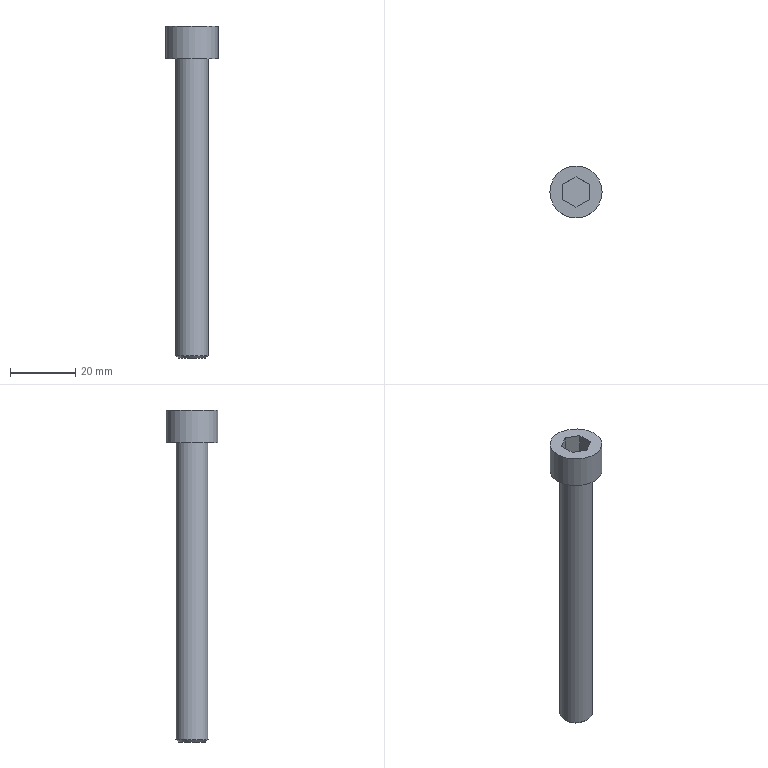Part | STEP file | gslz 2016.10.28-6_id902_x_t | 1 solid | 13 faces | box 16 x 16 x 102 mm | volume 8895 mm3 | plane 10 | cylinder 2 | cone 1 | commonest cylinder face diameters 10 x1 16 x1
STEP:
#1=CARTESIAN_POINT('',(60.7,151.843,72.));
#2=VERTEX_POINT('',#1);
#3=CARTESIAN_POINT('',(60.7,147.224,72.));
#4=VERTEX_POINT('',#3);
#5=CARTESIAN_POINT('',(60.7,151.843,72.));
#6=DIRECTION('',(0.,-1.,0.));
#7=VECTOR('',#6,1.);
#8=LINE('',#5,#7);
#9=EDGE_CURVE('',#2,#4,#8,.T.);
#10=ORIENTED_EDGE('',*,*,#9,.F.);
#11=CARTESIAN_POINT('',(64.7,154.152,72.));
#12=VERTEX_POINT('',#11);
#13=CARTESIAN_POINT('',(64.7,154.152,72.));
#14=DIRECTION('',(-0.866,-0.5,0.));
#15=VECTOR('',#14,1.);
#16=LINE('',#13,#15);
#17=EDGE_CURVE('',#12,#2,#16,.T.);
#18=ORIENTED_EDGE('',*,*,#17,.F.);
#19=CARTESIAN_POINT('',(68.7,151.843,72.));
#20=VERTEX_POINT('',#19);
#21=CARTESIAN_POINT('',(68.7,151.843,72.));
#22=DIRECTION('',(-0.866,0.5,0.));
#23=VECTOR('',#22,1.);
#24=LINE('',#21,#23);
#25=EDGE_CURVE('',#20,#12,#24,.T.);
#26=ORIENTED_EDGE('',*,*,#25,.F.);
#27=CARTESIAN_POINT('',(68.7,147.224,72.));
#28=VERTEX_POINT('',#27);
#29=CARTESIAN_POINT('',(68.7,147.224,72.));
#30=DIRECTION('',(0.,1.,0.));
#31=VECTOR('',#30,1.);
#32=LINE('',#29,#31);
#33=EDGE_CURVE('',#28,#20,#32,.T.);
#34=ORIENTED_EDGE('',*,*,#33,.F.);
#35=CARTESIAN_POINT('',(64.7,144.915,72.));
#36=VERTEX_POINT('',#35);
#37=CARTESIAN_POINT('',(64.7,144.915,72.));
#38=DIRECTION('',(0.866,0.5,0.));
#39=VECTOR('',#38,1.);
#40=LINE('',#37,#39);
#41=EDGE_CURVE('',#36,#28,#40,.T.);
#42=ORIENTED_EDGE('',*,*,#41,.F.);
#43=CARTESIAN_POINT('',(60.7,147.224,72.));
#44=DIRECTION('',(0.866,-0.5,0.));
#45=VECTOR('',#44,1.);
#46=LINE('',#43,#45);
#47=EDGE_CURVE('',#4,#36,#46,.T.);
#48=ORIENTED_EDGE('',*,*,#47,.F.);
#49=EDGE_LOOP('',(#10,#18,#26,#34,#42,#48));
#50=FACE_BOUND('',#49,.T.);
#51=CARTESIAN_POINT('',(72.7,149.533,72.));
#52=VERTEX_POINT('',#51);
#53=CARTESIAN_POINT('',(64.7,149.533,72.));
#54=DIRECTION('',(0.,0.,-1.));
#55=DIRECTION('',(1.,0.,0.));
#56=AXIS2_PLACEMENT_3D('',#53,#54,#55);
#57=CIRCLE('',#56,8.);
#58=EDGE_CURVE('',#52,#52,#57,.T.);
#59=ORIENTED_EDGE('',*,*,#58,.F.);
#60=EDGE_LOOP('',(#59));
#61=FACE_BOUND('',#60,.T.);
#62=CARTESIAN_POINT('',(64.7,149.533,72.));
#63=DIRECTION('',(0.,0.,1.));
#64=DIRECTION('',(-1.,0.,0.));
#65=AXIS2_PLACEMENT_3D('',#62,#63,#64);
#66=PLANE('',#65);
#67=ADVANCED_FACE('',(#50,#61),#66,.T.);
#68=CARTESIAN_POINT('',(60.45,149.533,-30.));
#69=VERTEX_POINT('',#68);
#70=CARTESIAN_POINT('',(64.7,149.533,-30.));
#71=DIRECTION('',(0.,0.,-1.));
#72=DIRECTION('',(-1.,0.,0.));
#73=AXIS2_PLACEMENT_3D('',#70,#71,#72);
#74=CIRCLE('',#73,4.25);
#75=EDGE_CURVE('',#69,#69,#74,.T.);
#76=ORIENTED_EDGE('',*,*,#75,.T.);
#77=EDGE_LOOP('',(#76));
#78=FACE_OUTER_BOUND('',#77,.T.);
#79=CARTESIAN_POINT('',(64.7,149.533,-30.));
#80=DIRECTION('',(0.,0.,-1.));
#81=DIRECTION('',(1.,0.,0.));
#82=AXIS2_PLACEMENT_3D('',#79,#80,#81);
#83=PLANE('',#82);
#84=ADVANCED_FACE('',(#78),#83,.T.);
#85=CARTESIAN_POINT('',(59.7,149.533,-29.25));
#86=VERTEX_POINT('',#85);
#87=CARTESIAN_POINT('',(64.7,149.533,-29.25));
#88=DIRECTION('',(0.,0.,1.));
#89=DIRECTION('',(-1.,0.,0.));
#90=AXIS2_PLACEMENT_3D('',#87,#88,#89);
#91=CIRCLE('',#90,5.);
#92=EDGE_CURVE('',#86,#86,#91,.T.);
#93=ORIENTED_EDGE('',*,*,#92,.T.);
#94=EDGE_LOOP('',(#93));
#95=FACE_BOUND('',#94,.T.);
#96=CARTESIAN_POINT('',(59.7,149.533,62.));
#97=VERTEX_POINT('',#96);
#98=CARTESIAN_POINT('',(64.7,149.533,62.));
#99=DIRECTION('',(0.,0.,-1.));
#100=DIRECTION('',(-1.,0.,0.));
#101=AXIS2_PLACEMENT_3D('',#98,#99,#100);
#102=CIRCLE('',#101,5.);
#103=EDGE_CURVE('',#97,#97,#102,.T.);
#104=ORIENTED_EDGE('',*,*,#103,.T.);
#105=EDGE_LOOP('',(#104));
#106=FACE_BOUND('',#105,.T.);
#107=CARTESIAN_POINT('',(64.7,149.533,-10.));
#108=DIRECTION('',(0.,0.,-1.));
#109=DIRECTION('',(-1.,0.,0.));
#110=AXIS2_PLACEMENT_3D('',#107,#108,#109);
#111=CYLINDRICAL_SURFACE('',#110,5.);
#112=ADVANCED_FACE('',(#95,#106),#111,.T.);
#113=ORIENTED_EDGE('',*,*,#103,.F.);
#114=EDGE_LOOP('',(#113));
#115=FACE_BOUND('',#114,.T.);
#116=CARTESIAN_POINT('',(56.7,149.533,62.));
#117=VERTEX_POINT('',#116);
#118=CARTESIAN_POINT('',(64.7,149.533,62.));
#119=DIRECTION('',(0.,0.,-1.));
#120=DIRECTION('',(-1.,0.,0.));
#121=AXIS2_PLACEMENT_3D('',#118,#119,#120);
#122=CIRCLE('',#121,8.);
#123=EDGE_CURVE('',#117,#117,#122,.T.);
#124=ORIENTED_EDGE('',*,*,#123,.T.);
#125=EDGE_LOOP('',(#124));
#126=FACE_BOUND('',#125,.T.);
#127=CARTESIAN_POINT('',(64.7,149.533,62.));
#128=DIRECTION('',(0.,0.,-1.));
#129=DIRECTION('',(1.,0.,0.));
#130=AXIS2_PLACEMENT_3D('',#127,#128,#129);
#131=PLANE('',#130);
#132=ADVANCED_FACE('',(#115,#126),#131,.T.);
#133=ORIENTED_EDGE('',*,*,#123,.F.);
#134=EDGE_LOOP('',(#133));
#135=FACE_BOUND('',#134,.T.);
#136=ORIENTED_EDGE('',*,*,#58,.T.);
#137=EDGE_LOOP('',(#136));
#138=FACE_BOUND('',#137,.T.);
#139=CARTESIAN_POINT('',(64.7,149.533,75.));
#140=DIRECTION('',(0.,0.,-1.));
#141=DIRECTION('',(-1.,0.,0.));
#142=AXIS2_PLACEMENT_3D('',#139,#140,#141);
#143=CYLINDRICAL_SURFACE('',#142,8.);
#144=ADVANCED_FACE('',(#135,#138),#143,.T.);
#145=ORIENTED_EDGE('',*,*,#9,.T.);
#146=CARTESIAN_POINT('',(60.7,147.224,66.));
#147=VERTEX_POINT('',#146);
#148=CARTESIAN_POINT('',(60.7,147.224,66.));
#149=DIRECTION('',(0.,0.,-1.));
#150=VECTOR('',#149,1.);
#151=LINE('',#148,#150);
#152=EDGE_CURVE('',#4,#147,#151,.T.);
#153=ORIENTED_EDGE('',*,*,#152,.T.);
#154=CARTESIAN_POINT('',(60.7,151.843,66.));
#155=VERTEX_POINT('',#154);
#156=CARTESIAN_POINT('',(60.7,151.843,66.));
#157=DIRECTION('',(0.,1.,0.));
#158=VECTOR('',#157,1.);
#159=LINE('',#156,#158);
#160=EDGE_CURVE('',#147,#155,#159,.T.);
#161=ORIENTED_EDGE('',*,*,#160,.T.);
#162=CARTESIAN_POINT('',(60.7,151.843,66.));
#163=DIRECTION('',(0.,0.,-1.));
#164=VECTOR('',#163,1.);
#165=LINE('',#162,#164);
#166=EDGE_CURVE('',#2,#155,#165,.T.);
#167=ORIENTED_EDGE('',*,*,#166,.F.);
#168=EDGE_LOOP('',(#145,#153,#161,#167));
#169=FACE_OUTER_BOUND('',#168,.T.);
#170=CARTESIAN_POINT('',(60.7,151.843,66.));
#171=DIRECTION('',(-1.,0.,0.));
#172=DIRECTION('',(0.,0.,1.));
#173=AXIS2_PLACEMENT_3D('',#170,#171,#172);
#174=PLANE('',#173);
#175=ADVANCED_FACE('',(#169),#174,.F.);
#176=ORIENTED_EDGE('',*,*,#47,.T.);
#177=CARTESIAN_POINT('',(64.7,144.915,66.));
#178=VERTEX_POINT('',#177);
#179=CARTESIAN_POINT('',(64.7,144.915,66.));
#180=DIRECTION('',(0.,0.,-1.));
#181=VECTOR('',#180,1.);
#182=LINE('',#179,#181);
#183=EDGE_CURVE('',#36,#178,#182,.T.);
#184=ORIENTED_EDGE('',*,*,#183,.T.);
#185=CARTESIAN_POINT('',(60.7,147.224,66.));
#186=DIRECTION('',(-0.866,0.5,0.));
#187=VECTOR('',#186,1.);
#188=LINE('',#185,#187);
#189=EDGE_CURVE('',#178,#147,#188,.T.);
#190=ORIENTED_EDGE('',*,*,#189,.T.);
#191=ORIENTED_EDGE('',*,*,#152,.F.);
#192=EDGE_LOOP('',(#176,#184,#190,#191));
#193=FACE_OUTER_BOUND('',#192,.T.);
#194=CARTESIAN_POINT('',(60.7,147.224,66.));
#195=DIRECTION('',(-0.5,-0.866,0.));
#196=DIRECTION('',(-0.866,0.5,0.));
#197=AXIS2_PLACEMENT_3D('',#194,#195,#196);
#198=PLANE('',#197);
#199=ADVANCED_FACE('',(#193),#198,.F.);
#200=ORIENTED_EDGE('',*,*,#41,.T.);
#201=CARTESIAN_POINT('',(68.7,147.224,66.));
#202=VERTEX_POINT('',#201);
#203=CARTESIAN_POINT('',(68.7,147.224,66.));
#204=DIRECTION('',(0.,0.,-1.));
#205=VECTOR('',#204,1.);
#206=LINE('',#203,#205);
#207=EDGE_CURVE('',#28,#202,#206,.T.);
#208=ORIENTED_EDGE('',*,*,#207,.T.);
#209=CARTESIAN_POINT('',(64.7,144.915,66.));
#210=DIRECTION('',(-0.866,-0.5,0.));
#211=VECTOR('',#210,1.);
#212=LINE('',#209,#211);
#213=EDGE_CURVE('',#202,#178,#212,.T.);
#214=ORIENTED_EDGE('',*,*,#213,.T.);
#215=ORIENTED_EDGE('',*,*,#183,.F.);
#216=EDGE_LOOP('',(#200,#208,#214,#215));
#217=FACE_OUTER_BOUND('',#216,.T.);
#218=CARTESIAN_POINT('',(64.7,144.915,66.));
#219=DIRECTION('',(0.5,-0.866,0.));
#220=DIRECTION('',(-0.866,-0.5,0.));
#221=AXIS2_PLACEMENT_3D('',#218,#219,#220);
#222=PLANE('',#221);
#223=ADVANCED_FACE('',(#217),#222,.F.);
#224=ORIENTED_EDGE('',*,*,#33,.T.);
#225=CARTESIAN_POINT('',(68.7,151.843,66.));
#226=VERTEX_POINT('',#225);
#227=CARTESIAN_POINT('',(68.7,151.843,66.));
#228=DIRECTION('',(0.,0.,-1.));
#229=VECTOR('',#228,1.);
#230=LINE('',#227,#229);
#231=EDGE_CURVE('',#20,#226,#230,.T.);
#232=ORIENTED_EDGE('',*,*,#231,.T.);
#233=CARTESIAN_POINT('',(68.7,147.224,66.));
#234=DIRECTION('',(0.,-1.,0.));
#235=VECTOR('',#234,1.);
#236=LINE('',#233,#235);
#237=EDGE_CURVE('',#226,#202,#236,.T.);
#238=ORIENTED_EDGE('',*,*,#237,.T.);
#239=ORIENTED_EDGE('',*,*,#207,.F.);
#240=EDGE_LOOP('',(#224,#232,#238,#239));
#241=FACE_OUTER_BOUND('',#240,.T.);
#242=CARTESIAN_POINT('',(68.7,147.224,66.));
#243=DIRECTION('',(1.,0.,0.));
#244=DIRECTION('',(0.,0.,1.));
#245=AXIS2_PLACEMENT_3D('',#242,#243,#244);
#246=PLANE('',#245);
#247=ADVANCED_FACE('',(#241),#246,.F.);
#248=ORIENTED_EDGE('',*,*,#25,.T.);
#249=CARTESIAN_POINT('',(64.7,154.152,66.));
#250=VERTEX_POINT('',#249);
#251=CARTESIAN_POINT('',(64.7,154.152,66.));
#252=DIRECTION('',(0.,0.,-1.));
#253=VECTOR('',#252,1.);
#254=LINE('',#251,#253);
#255=EDGE_CURVE('',#12,#250,#254,.T.);
#256=ORIENTED_EDGE('',*,*,#255,.T.);
#257=CARTESIAN_POINT('',(68.7,151.843,66.));
#258=DIRECTION('',(0.866,-0.5,0.));
#259=VECTOR('',#258,1.);
#260=LINE('',#257,#259);
#261=EDGE_CURVE('',#250,#226,#260,.T.);
#262=ORIENTED_EDGE('',*,*,#261,.T.);
#263=ORIENTED_EDGE('',*,*,#231,.F.);
#264=EDGE_LOOP('',(#248,#256,#262,#263));
#265=FACE_OUTER_BOUND('',#264,.T.);
#266=CARTESIAN_POINT('',(68.7,151.843,66.));
#267=DIRECTION('',(0.5,0.866,0.));
#268=DIRECTION('',(0.866,-0.5,0.));
#269=AXIS2_PLACEMENT_3D('',#266,#267,#268);
#270=PLANE('',#269);
#271=ADVANCED_FACE('',(#265),#270,.F.);
#272=ORIENTED_EDGE('',*,*,#17,.T.);
#273=ORIENTED_EDGE('',*,*,#166,.T.);
#274=CARTESIAN_POINT('',(64.7,154.152,66.));
#275=DIRECTION('',(0.866,0.5,0.));
#276=VECTOR('',#275,1.);
#277=LINE('',#274,#276);
#278=EDGE_CURVE('',#155,#250,#277,.T.);
#279=ORIENTED_EDGE('',*,*,#278,.T.);
#280=ORIENTED_EDGE('',*,*,#255,.F.);
#281=EDGE_LOOP('',(#272,#273,#279,#280));
#282=FACE_OUTER_BOUND('',#281,.T.);
#283=CARTESIAN_POINT('',(64.7,154.152,66.));
#284=DIRECTION('',(-0.5,0.866,0.));
#285=DIRECTION('',(0.866,0.5,0.));
#286=AXIS2_PLACEMENT_3D('',#283,#284,#285);
#287=PLANE('',#286);
#288=ADVANCED_FACE('',(#282),#287,.F.);
#289=ORIENTED_EDGE('',*,*,#160,.F.);
#290=ORIENTED_EDGE('',*,*,#189,.F.);
#291=ORIENTED_EDGE('',*,*,#213,.F.);
#292=ORIENTED_EDGE('',*,*,#237,.F.);
#293=ORIENTED_EDGE('',*,*,#261,.F.);
#294=ORIENTED_EDGE('',*,*,#278,.F.);
#295=EDGE_LOOP('',(#289,#290,#291,#292,#293,#294));
#296=FACE_OUTER_BOUND('',#295,.T.);
#297=CARTESIAN_POINT('',(60.7,147.224,66.));
#298=DIRECTION('',(0.,0.,1.));
#299=DIRECTION('',(-1.,0.,0.));
#300=AXIS2_PLACEMENT_3D('',#297,#298,#299);
#301=PLANE('',#300);
#302=ADVANCED_FACE('',(#296),#301,.T.);
#303=ORIENTED_EDGE('',*,*,#92,.F.);
#304=EDGE_LOOP('',(#303));
#305=FACE_BOUND('',#304,.T.);
#306=ORIENTED_EDGE('',*,*,#75,.F.);
#307=EDGE_LOOP('',(#306));
#308=FACE_BOUND('',#307,.T.);
#309=CARTESIAN_POINT('',(64.7,149.533,-30.));
#310=DIRECTION('',(0.,0.,1.));
#311=DIRECTION('',(1.,0.,0.));
#312=AXIS2_PLACEMENT_3D('',#309,#310,#311);
#313=CONICAL_SURFACE('',#312,4.25,45.);
#314=ADVANCED_FACE('',(#305,#308),#313,.T.);
#315=CLOSED_SHELL('',(#67,#84,#112,#132,#144,#175,#199,#223,#247,#271,#288,#302,#314));
#316=MANIFOLD_SOLID_BREP('',#315);
#317=(LENGTH_UNIT()NAMED_UNIT(*)SI_UNIT(.MILLI.,.METRE.));
#318=UNCERTAINTY_MEASURE_WITH_UNIT(LENGTH_MEASURE(0.00002),#317,'','');
#319=(NAMED_UNIT(*)PLANE_ANGLE_UNIT()SI_UNIT($,.RADIAN.));
#320=PLANE_ANGLE_MEASURE_WITH_UNIT(PLANE_ANGLE_MEASURE(0.01745),#319);
#321=DIMENSIONAL_EXPONENTS(0.,0.,0.,0.,0.,0.,0.);
#322=(CONVERSION_BASED_UNIT('DEGREE',#320)NAMED_UNIT(#321)PLANE_ANGLE_UNIT());
#323=(NAMED_UNIT(*)SI_UNIT($,.STERADIAN.)SOLID_ANGLE_UNIT());
#324=(GEOMETRIC_REPRESENTATION_CONTEXT(3)GLOBAL_UNCERTAINTY_ASSIGNED_CONTEXT((#318))GLOBAL_UNIT_ASSIGNED_CONTEXT((#317,#322,#323))REPRESENTATION_CONTEXT('',''));
#325=ADVANCED_BREP_SHAPE_REPRESENTATION('',(#316),#324);